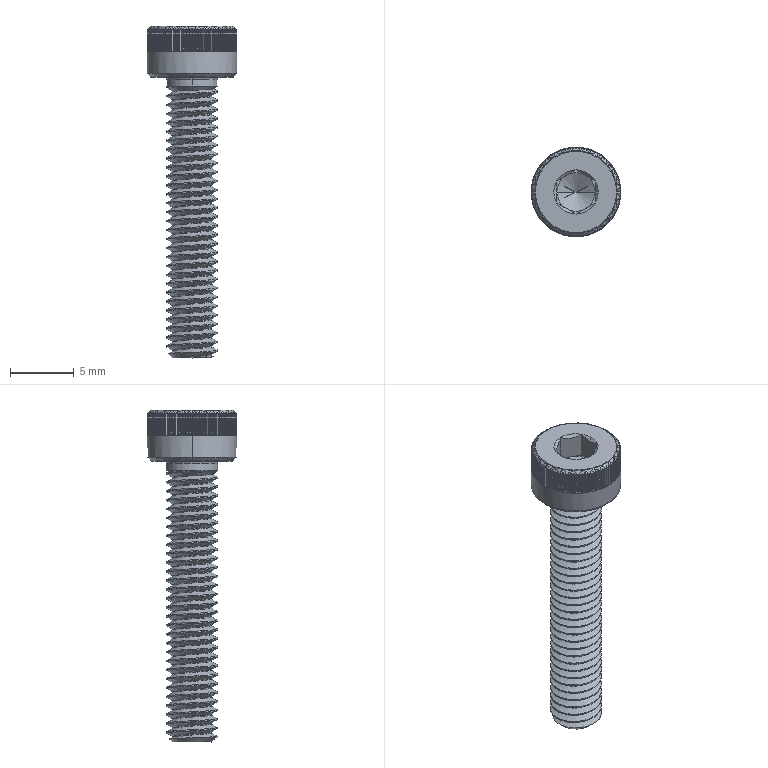Part | NX | features solid 2 | 1 solid | 1873 faces | box 7 x 7 x 26 mm | volume 353.505 mm3 | spline 983 | cylinder 357 | plane 211 | torus 205 | cone 117 | commonest cylinder face diameters 0.025 x196 0.018 x98 4 x61 7 x2